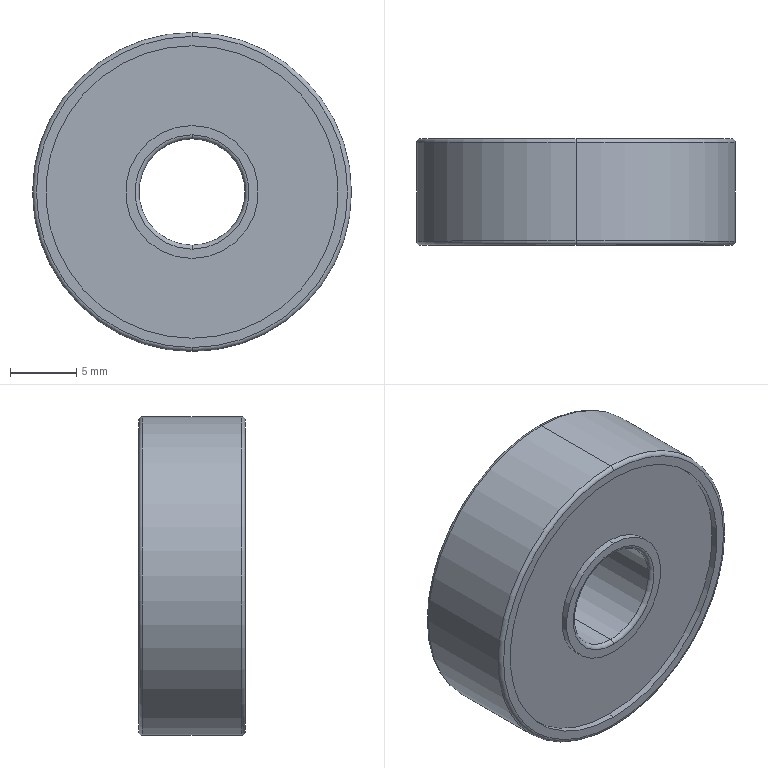Part | STEP file | Domestic miniature ball bearing NSK 628ZZ-1 | 1 solid | 26 faces | box 24 x 8 x 24 mm | volume 2912 mm3 | cylinder 12 | torus 8 | plane 6 | commonest cylinder face diameters 10 x4 22 x4 8 x2 24 x2
STEP:
#1=CARTESIAN_POINT('',(0.,24.998,-12.));
#2=VERTEX_POINT('',#1);
#3=CARTESIAN_POINT('',(0.,24.998,12.));
#4=VERTEX_POINT('',#3);
#5=CARTESIAN_POINT('',(0.,24.998,0.));
#6=DIRECTION('',(0.,-1.,0.));
#7=DIRECTION('',(0.,0.,1.));
#8=AXIS2_PLACEMENT_3D('',#5,#6,#7);
#9=CIRCLE('',#8,12.);
#10=EDGE_CURVE('',#2,#4,#9,.T.);
#11=ORIENTED_EDGE('',*,*,#10,.F.);
#12=CARTESIAN_POINT('',(0.,25.298,-11.7));
#13=VERTEX_POINT('',#12);
#14=CARTESIAN_POINT('',(0.,24.998,-11.7));
#15=DIRECTION('',(1.,0.,0.));
#16=DIRECTION('',(0.,0.,-1.));
#17=AXIS2_PLACEMENT_3D('',#14,#15,#16);
#18=CIRCLE('',#17,0.3);
#19=EDGE_CURVE('',#2,#13,#18,.T.);
#20=ORIENTED_EDGE('',*,*,#19,.T.);
#21=CARTESIAN_POINT('',(0.,25.298,11.7));
#22=VERTEX_POINT('',#21);
#23=CARTESIAN_POINT('',(0.,25.298,0.));
#24=DIRECTION('',(0.,1.,0.));
#25=DIRECTION('',(0.,0.,1.));
#26=AXIS2_PLACEMENT_3D('',#23,#24,#25);
#27=CIRCLE('',#26,11.7);
#28=EDGE_CURVE('',#22,#13,#27,.T.);
#29=ORIENTED_EDGE('',*,*,#28,.F.);
#30=CARTESIAN_POINT('',(0.,24.998,11.7));
#31=DIRECTION('',(-1.,0.,0.));
#32=DIRECTION('',(0.,0.,1.));
#33=AXIS2_PLACEMENT_3D('',#30,#31,#32);
#34=CIRCLE('',#33,0.3);
#35=EDGE_CURVE('',#4,#22,#34,.T.);
#36=ORIENTED_EDGE('',*,*,#35,.F.);
#37=EDGE_LOOP('',(#11,#20,#29,#36));
#38=FACE_OUTER_BOUND('',#37,.T.);
#39=CARTESIAN_POINT('',(0.,24.998,0.));
#40=DIRECTION('',(0.,1.,0.));
#41=DIRECTION('',(0.,0.,1.));
#42=AXIS2_PLACEMENT_3D('',#39,#40,#41);
#43=TOROIDAL_SURFACE('',#42,11.7,0.3);
#44=ADVANCED_FACE('',(#38),#43,.T.);
#45=CARTESIAN_POINT('',(0.,17.598,12.));
#46=VERTEX_POINT('',#45);
#47=CARTESIAN_POINT('',(0.,17.598,-12.));
#48=VERTEX_POINT('',#47);
#49=CARTESIAN_POINT('',(0.,17.598,0.));
#50=DIRECTION('',(0.,1.,0.));
#51=DIRECTION('',(0.,0.,-1.));
#52=AXIS2_PLACEMENT_3D('',#49,#50,#51);
#53=CIRCLE('',#52,12.);
#54=EDGE_CURVE('',#46,#48,#53,.T.);
#55=ORIENTED_EDGE('',*,*,#54,.F.);
#56=CARTESIAN_POINT('',(0.,17.298,11.7));
#57=VERTEX_POINT('',#56);
#58=CARTESIAN_POINT('',(0.,17.598,11.7));
#59=DIRECTION('',(1.,0.,0.));
#60=DIRECTION('',(0.,0.,-1.));
#61=AXIS2_PLACEMENT_3D('',#58,#59,#60);
#62=CIRCLE('',#61,0.3);
#63=EDGE_CURVE('',#46,#57,#62,.T.);
#64=ORIENTED_EDGE('',*,*,#63,.T.);
#65=CARTESIAN_POINT('',(0.,17.298,-11.7));
#66=VERTEX_POINT('',#65);
#67=CARTESIAN_POINT('',(0.,17.298,0.));
#68=DIRECTION('',(0.,-1.,0.));
#69=DIRECTION('',(0.,0.,-1.));
#70=AXIS2_PLACEMENT_3D('',#67,#68,#69);
#71=CIRCLE('',#70,11.7);
#72=EDGE_CURVE('',#66,#57,#71,.T.);
#73=ORIENTED_EDGE('',*,*,#72,.F.);
#74=CARTESIAN_POINT('',(0.,17.598,-11.7));
#75=DIRECTION('',(-1.,0.,0.));
#76=DIRECTION('',(0.,0.,1.));
#77=AXIS2_PLACEMENT_3D('',#74,#75,#76);
#78=CIRCLE('',#77,0.3);
#79=EDGE_CURVE('',#48,#66,#78,.T.);
#80=ORIENTED_EDGE('',*,*,#79,.F.);
#81=EDGE_LOOP('',(#55,#64,#73,#80));
#82=FACE_OUTER_BOUND('',#81,.T.);
#83=CARTESIAN_POINT('',(0.,17.598,0.));
#84=DIRECTION('',(0.,-1.,0.));
#85=DIRECTION('',(0.,0.,-1.));
#86=AXIS2_PLACEMENT_3D('',#83,#84,#85);
#87=TOROIDAL_SURFACE('',#86,11.7,0.3);
#88=ADVANCED_FACE('',(#82),#87,.T.);
#89=CARTESIAN_POINT('',(0.,25.298,-4.3));
#90=VERTEX_POINT('',#89);
#91=CARTESIAN_POINT('',(0.,25.298,4.3));
#92=VERTEX_POINT('',#91);
#93=CARTESIAN_POINT('',(0.,25.298,0.));
#94=DIRECTION('',(0.,-1.,0.));
#95=DIRECTION('',(0.,0.,1.));
#96=AXIS2_PLACEMENT_3D('',#93,#94,#95);
#97=CIRCLE('',#96,4.3);
#98=EDGE_CURVE('',#90,#92,#97,.T.);
#99=ORIENTED_EDGE('',*,*,#98,.F.);
#100=CARTESIAN_POINT('',(0.,24.998,-4.));
#101=VERTEX_POINT('',#100);
#102=CARTESIAN_POINT('',(0.,24.998,-4.3));
#103=DIRECTION('',(1.,0.,0.));
#104=DIRECTION('',(0.,0.,-1.));
#105=AXIS2_PLACEMENT_3D('',#102,#103,#104);
#106=CIRCLE('',#105,0.3);
#107=EDGE_CURVE('',#90,#101,#106,.T.);
#108=ORIENTED_EDGE('',*,*,#107,.T.);
#109=CARTESIAN_POINT('',(0.,24.998,4.));
#110=VERTEX_POINT('',#109);
#111=CARTESIAN_POINT('',(0.,24.998,0.));
#112=DIRECTION('',(0.,1.,0.));
#113=DIRECTION('',(0.,0.,1.));
#114=AXIS2_PLACEMENT_3D('',#111,#112,#113);
#115=CIRCLE('',#114,4.);
#116=EDGE_CURVE('',#110,#101,#115,.T.);
#117=ORIENTED_EDGE('',*,*,#116,.F.);
#118=CARTESIAN_POINT('',(0.,24.998,4.3));
#119=DIRECTION('',(-1.,0.,0.));
#120=DIRECTION('',(0.,0.,1.));
#121=AXIS2_PLACEMENT_3D('',#118,#119,#120);
#122=CIRCLE('',#121,0.3);
#123=EDGE_CURVE('',#92,#110,#122,.T.);
#124=ORIENTED_EDGE('',*,*,#123,.F.);
#125=EDGE_LOOP('',(#99,#108,#117,#124));
#126=FACE_OUTER_BOUND('',#125,.T.);
#127=CARTESIAN_POINT('',(0.,24.998,0.));
#128=DIRECTION('',(0.,1.,0.));
#129=DIRECTION('',(0.,0.,1.));
#130=AXIS2_PLACEMENT_3D('',#127,#128,#129);
#131=TOROIDAL_SURFACE('',#130,4.3,0.3);
#132=ADVANCED_FACE('',(#126),#131,.T.);
#133=CARTESIAN_POINT('',(0.,17.298,4.3));
#134=VERTEX_POINT('',#133);
#135=CARTESIAN_POINT('',(0.,17.298,-4.3));
#136=VERTEX_POINT('',#135);
#137=CARTESIAN_POINT('',(0.,17.298,0.));
#138=DIRECTION('',(0.,1.,0.));
#139=DIRECTION('',(0.,0.,-1.));
#140=AXIS2_PLACEMENT_3D('',#137,#138,#139);
#141=CIRCLE('',#140,4.3);
#142=EDGE_CURVE('',#134,#136,#141,.T.);
#143=ORIENTED_EDGE('',*,*,#142,.F.);
#144=CARTESIAN_POINT('',(0.,17.598,4.));
#145=VERTEX_POINT('',#144);
#146=CARTESIAN_POINT('',(0.,17.598,4.3));
#147=DIRECTION('',(1.,0.,0.));
#148=DIRECTION('',(0.,0.,-1.));
#149=AXIS2_PLACEMENT_3D('',#146,#147,#148);
#150=CIRCLE('',#149,0.3);
#151=EDGE_CURVE('',#134,#145,#150,.T.);
#152=ORIENTED_EDGE('',*,*,#151,.T.);
#153=CARTESIAN_POINT('',(0.,17.598,-4.));
#154=VERTEX_POINT('',#153);
#155=CARTESIAN_POINT('',(0.,17.598,0.));
#156=DIRECTION('',(0.,-1.,0.));
#157=DIRECTION('',(0.,0.,-1.));
#158=AXIS2_PLACEMENT_3D('',#155,#156,#157);
#159=CIRCLE('',#158,4.);
#160=EDGE_CURVE('',#154,#145,#159,.T.);
#161=ORIENTED_EDGE('',*,*,#160,.F.);
#162=CARTESIAN_POINT('',(0.,17.598,-4.3));
#163=DIRECTION('',(-1.,0.,0.));
#164=DIRECTION('',(0.,0.,1.));
#165=AXIS2_PLACEMENT_3D('',#162,#163,#164);
#166=CIRCLE('',#165,0.3);
#167=EDGE_CURVE('',#136,#154,#166,.T.);
#168=ORIENTED_EDGE('',*,*,#167,.F.);
#169=EDGE_LOOP('',(#143,#152,#161,#168));
#170=FACE_OUTER_BOUND('',#169,.T.);
#171=CARTESIAN_POINT('',(0.,17.598,0.));
#172=DIRECTION('',(0.,-1.,0.));
#173=DIRECTION('',(0.,0.,-1.));
#174=AXIS2_PLACEMENT_3D('',#171,#172,#173);
#175=TOROIDAL_SURFACE('',#174,4.3,0.3);
#176=ADVANCED_FACE('',(#170),#175,.T.);
#177=CARTESIAN_POINT('',(0.,25.298,-5.));
#178=VERTEX_POINT('',#177);
#179=CARTESIAN_POINT('',(0.,25.298,5.));
#180=VERTEX_POINT('',#179);
#181=CARTESIAN_POINT('',(0.,25.298,0.));
#182=DIRECTION('',(0.,-1.,0.));
#183=DIRECTION('',(0.,0.,-1.));
#184=AXIS2_PLACEMENT_3D('',#181,#182,#183);
#185=CIRCLE('',#184,5.);
#186=EDGE_CURVE('',#178,#180,#185,.T.);
#187=ORIENTED_EDGE('',*,*,#186,.T.);
#188=CARTESIAN_POINT('',(0.,24.798,5.));
#189=VERTEX_POINT('',#188);
#190=CARTESIAN_POINT('',(0.,0.,5.));
#191=DIRECTION('',(0.,-1.,0.));
#192=VECTOR('',#191,1000.);
#193=LINE('',#190,#192);
#194=EDGE_CURVE('',#180,#189,#193,.T.);
#195=ORIENTED_EDGE('',*,*,#194,.T.);
#196=CARTESIAN_POINT('',(0.,24.798,-5.));
#197=VERTEX_POINT('',#196);
#198=CARTESIAN_POINT('',(0.,24.798,0.));
#199=DIRECTION('',(0.,-1.,0.));
#200=DIRECTION('',(0.,0.,-1.));
#201=AXIS2_PLACEMENT_3D('',#198,#199,#200);
#202=CIRCLE('',#201,5.);
#203=EDGE_CURVE('',#197,#189,#202,.T.);
#204=ORIENTED_EDGE('',*,*,#203,.F.);
#205=CARTESIAN_POINT('',(0.,0.,-5.));
#206=DIRECTION('',(0.,-1.,0.));
#207=VECTOR('',#206,1000.);
#208=LINE('',#205,#207);
#209=EDGE_CURVE('',#178,#197,#208,.T.);
#210=ORIENTED_EDGE('',*,*,#209,.F.);
#211=EDGE_LOOP('',(#187,#195,#204,#210));
#212=FACE_OUTER_BOUND('',#211,.T.);
#213=CARTESIAN_POINT('',(0.,0.,0.));
#214=DIRECTION('',(0.,-1.,0.));
#215=DIRECTION('',(0.,0.,-1.));
#216=AXIS2_PLACEMENT_3D('',#213,#214,#215);
#217=CYLINDRICAL_SURFACE('',#216,5.);
#218=ADVANCED_FACE('',(#212),#217,.T.);
#219=CARTESIAN_POINT('',(0.,25.298,11.));
#220=VERTEX_POINT('',#219);
#221=CARTESIAN_POINT('',(0.,25.298,-11.));
#222=VERTEX_POINT('',#221);
#223=CARTESIAN_POINT('',(0.,25.298,0.));
#224=DIRECTION('',(0.,-1.,0.));
#225=DIRECTION('',(0.,0.,-1.));
#226=AXIS2_PLACEMENT_3D('',#223,#224,#225);
#227=CIRCLE('',#226,11.);
#228=EDGE_CURVE('',#220,#222,#227,.T.);
#229=ORIENTED_EDGE('',*,*,#228,.F.);
#230=CARTESIAN_POINT('',(0.,24.798,11.));
#231=VERTEX_POINT('',#230);
#232=CARTESIAN_POINT('',(0.,0.,11.));
#233=DIRECTION('',(0.,-1.,0.));
#234=VECTOR('',#233,1000.);
#235=LINE('',#232,#234);
#236=EDGE_CURVE('',#220,#231,#235,.T.);
#237=ORIENTED_EDGE('',*,*,#236,.T.);
#238=CARTESIAN_POINT('',(0.,24.798,-11.));
#239=VERTEX_POINT('',#238);
#240=CARTESIAN_POINT('',(0.,24.798,0.));
#241=DIRECTION('',(0.,-1.,0.));
#242=DIRECTION('',(0.,0.,-1.));
#243=AXIS2_PLACEMENT_3D('',#240,#241,#242);
#244=CIRCLE('',#243,11.);
#245=EDGE_CURVE('',#231,#239,#244,.T.);
#246=ORIENTED_EDGE('',*,*,#245,.T.);
#247=CARTESIAN_POINT('',(0.,0.,-11.));
#248=DIRECTION('',(0.,-1.,0.));
#249=VECTOR('',#248,1000.);
#250=LINE('',#247,#249);
#251=EDGE_CURVE('',#222,#239,#250,.T.);
#252=ORIENTED_EDGE('',*,*,#251,.F.);
#253=EDGE_LOOP('',(#229,#237,#246,#252));
#254=FACE_OUTER_BOUND('',#253,.T.);
#255=CARTESIAN_POINT('',(0.,0.,0.));
#256=DIRECTION('',(0.,-1.,0.));
#257=DIRECTION('',(0.,0.,-1.));
#258=AXIS2_PLACEMENT_3D('',#255,#256,#257);
#259=CYLINDRICAL_SURFACE('',#258,11.);
#260=ADVANCED_FACE('',(#254),#259,.F.);
#261=ORIENTED_EDGE('',*,*,#10,.T.);
#262=CARTESIAN_POINT('',(0.,0.,12.));
#263=DIRECTION('',(0.,-1.,0.));
#264=VECTOR('',#263,1000.);
#265=LINE('',#262,#264);
#266=EDGE_CURVE('',#4,#46,#265,.T.);
#267=ORIENTED_EDGE('',*,*,#266,.T.);
#268=ORIENTED_EDGE('',*,*,#54,.T.);
#269=CARTESIAN_POINT('',(0.,0.,-12.));
#270=DIRECTION('',(0.,-1.,0.));
#271=VECTOR('',#270,1000.);
#272=LINE('',#269,#271);
#273=EDGE_CURVE('',#2,#48,#272,.T.);
#274=ORIENTED_EDGE('',*,*,#273,.F.);
#275=EDGE_LOOP('',(#261,#267,#268,#274));
#276=FACE_OUTER_BOUND('',#275,.T.);
#277=CARTESIAN_POINT('',(0.,0.,0.));
#278=DIRECTION('',(0.,-1.,0.));
#279=DIRECTION('',(0.,0.,-1.));
#280=AXIS2_PLACEMENT_3D('',#277,#278,#279);
#281=CYLINDRICAL_SURFACE('',#280,12.);
#282=ADVANCED_FACE('',(#276),#281,.T.);
#283=CARTESIAN_POINT('',(0.,17.798,11.));
#284=VERTEX_POINT('',#283);
#285=CARTESIAN_POINT('',(0.,17.798,-11.));
#286=VERTEX_POINT('',#285);
#287=CARTESIAN_POINT('',(0.,17.798,0.));
#288=DIRECTION('',(0.,-1.,0.));
#289=DIRECTION('',(0.,0.,-1.));
#290=AXIS2_PLACEMENT_3D('',#287,#288,#289);
#291=CIRCLE('',#290,11.);
#292=EDGE_CURVE('',#284,#286,#291,.T.);
#293=ORIENTED_EDGE('',*,*,#292,.F.);
#294=CARTESIAN_POINT('',(0.,17.298,11.));
#295=VERTEX_POINT('',#294);
#296=CARTESIAN_POINT('',(0.,0.,11.));
#297=DIRECTION('',(0.,-1.,0.));
#298=VECTOR('',#297,1000.);
#299=LINE('',#296,#298);
#300=EDGE_CURVE('',#284,#295,#299,.T.);
#301=ORIENTED_EDGE('',*,*,#300,.T.);
#302=CARTESIAN_POINT('',(0.,17.298,-11.));
#303=VERTEX_POINT('',#302);
#304=CARTESIAN_POINT('',(0.,17.298,0.));
#305=DIRECTION('',(0.,-1.,0.));
#306=DIRECTION('',(0.,0.,-1.));
#307=AXIS2_PLACEMENT_3D('',#304,#305,#306);
#308=CIRCLE('',#307,11.);
#309=EDGE_CURVE('',#295,#303,#308,.T.);
#310=ORIENTED_EDGE('',*,*,#309,.T.);
#311=CARTESIAN_POINT('',(0.,0.,-11.));
#312=DIRECTION('',(0.,-1.,0.));
#313=VECTOR('',#312,1000.);
#314=LINE('',#311,#313);
#315=EDGE_CURVE('',#286,#303,#314,.T.);
#316=ORIENTED_EDGE('',*,*,#315,.F.);
#317=EDGE_LOOP('',(#293,#301,#310,#316));
#318=FACE_OUTER_BOUND('',#317,.T.);
#319=CARTESIAN_POINT('',(0.,0.,0.));
#320=DIRECTION('',(0.,-1.,0.));
#321=DIRECTION('',(0.,0.,-1.));
#322=AXIS2_PLACEMENT_3D('',#319,#320,#321);
#323=CYLINDRICAL_SURFACE('',#322,11.);
#324=ADVANCED_FACE('',(#318),#323,.F.);
#325=CARTESIAN_POINT('',(0.,17.798,-5.));
#326=VERTEX_POINT('',#325);
#327=CARTESIAN_POINT('',(0.,17.798,5.));
#328=VERTEX_POINT('',#327);
#329=CARTESIAN_POINT('',(0.,17.798,0.));
#330=DIRECTION('',(0.,-1.,0.));
#331=DIRECTION('',(0.,0.,-1.));
#332=AXIS2_PLACEMENT_3D('',#329,#330,#331);
#333=CIRCLE('',#332,5.);
#334=EDGE_CURVE('',#326,#328,#333,.T.);
#335=ORIENTED_EDGE('',*,*,#334,.T.);
#336=CARTESIAN_POINT('',(0.,17.298,5.));
#337=VERTEX_POINT('',#336);
#338=CARTESIAN_POINT('',(0.,0.,5.));
#339=DIRECTION('',(0.,-1.,0.));
#340=VECTOR('',#339,1000.);
#341=LINE('',#338,#340);
#342=EDGE_CURVE('',#328,#337,#341,.T.);
#343=ORIENTED_EDGE('',*,*,#342,.T.);
#344=CARTESIAN_POINT('',(0.,17.298,-5.));
#345=VERTEX_POINT('',#344);
#346=CARTESIAN_POINT('',(0.,17.298,0.));
#347=DIRECTION('',(0.,-1.,0.));
#348=DIRECTION('',(0.,0.,-1.));
#349=AXIS2_PLACEMENT_3D('',#346,#347,#348);
#350=CIRCLE('',#349,5.);
#351=EDGE_CURVE('',#345,#337,#350,.T.);
#352=ORIENTED_EDGE('',*,*,#351,.F.);
#353=CARTESIAN_POINT('',(0.,0.,-5.));
#354=DIRECTION('',(0.,-1.,0.));
#355=VECTOR('',#354,1000.);
#356=LINE('',#353,#355);
#357=EDGE_CURVE('',#326,#345,#356,.T.);
#358=ORIENTED_EDGE('',*,*,#357,.F.);
#359=EDGE_LOOP('',(#335,#343,#352,#358));
#360=FACE_OUTER_BOUND('',#359,.T.);
#361=CARTESIAN_POINT('',(0.,0.,0.));
#362=DIRECTION('',(0.,-1.,0.));
#363=DIRECTION('',(0.,0.,-1.));
#364=AXIS2_PLACEMENT_3D('',#361,#362,#363);
#365=CYLINDRICAL_SURFACE('',#364,5.);
#366=ADVANCED_FACE('',(#360),#365,.T.);
#367=CARTESIAN_POINT('',(0.,24.998,0.));
#368=DIRECTION('',(0.,1.,0.));
#369=DIRECTION('',(0.,0.,1.));
#370=AXIS2_PLACEMENT_3D('',#367,#368,#369);
#371=CIRCLE('',#370,4.);
#372=EDGE_CURVE('',#101,#110,#371,.T.);
#373=ORIENTED_EDGE('',*,*,#372,.T.);
#374=CARTESIAN_POINT('',(0.,0.,4.));
#375=DIRECTION('',(0.,-1.,0.));
#376=VECTOR('',#375,1000.);
#377=LINE('',#374,#376);
#378=EDGE_CURVE('',#110,#145,#377,.T.);
#379=ORIENTED_EDGE('',*,*,#378,.T.);
#380=CARTESIAN_POINT('',(0.,17.598,0.));
#381=DIRECTION('',(0.,-1.,0.));
#382=DIRECTION('',(0.,0.,-1.));
#383=AXIS2_PLACEMENT_3D('',#380,#381,#382);
#384=CIRCLE('',#383,4.);
#385=EDGE_CURVE('',#145,#154,#384,.T.);
#386=ORIENTED_EDGE('',*,*,#385,.T.);
#387=CARTESIAN_POINT('',(0.,0.,-4.));
#388=DIRECTION('',(0.,-1.,0.));
#389=VECTOR('',#388,1000.);
#390=LINE('',#387,#389);
#391=EDGE_CURVE('',#101,#154,#390,.T.);
#392=ORIENTED_EDGE('',*,*,#391,.F.);
#393=EDGE_LOOP('',(#373,#379,#386,#392));
#394=FACE_OUTER_BOUND('',#393,.T.);
#395=CARTESIAN_POINT('',(0.,0.,0.));
#396=DIRECTION('',(0.,-1.,0.));
#397=DIRECTION('',(0.,0.,-1.));
#398=AXIS2_PLACEMENT_3D('',#395,#396,#397);
#399=CYLINDRICAL_SURFACE('',#398,4.);
#400=ADVANCED_FACE('',(#394),#399,.F.);
#401=CARTESIAN_POINT('',(0.,25.298,0.));
#402=DIRECTION('',(0.,-1.,0.));
#403=DIRECTION('',(0.,0.,1.));
#404=AXIS2_PLACEMENT_3D('',#401,#402,#403);
#405=CIRCLE('',#404,4.3);
#406=EDGE_CURVE('',#92,#90,#405,.T.);
#407=ORIENTED_EDGE('',*,*,#406,.T.);
#408=ORIENTED_EDGE('',*,*,#98,.T.);
#409=EDGE_LOOP('',(#407,#408));
#410=FACE_BOUND('',#409,.T.);
#411=ORIENTED_EDGE('',*,*,#186,.F.);
#412=CARTESIAN_POINT('',(0.,25.298,0.));
#413=DIRECTION('',(0.,-1.,0.));
#414=DIRECTION('',(0.,0.,-1.));
#415=AXIS2_PLACEMENT_3D('',#412,#413,#414);
#416=CIRCLE('',#415,5.);
#417=EDGE_CURVE('',#180,#178,#416,.T.);
#418=ORIENTED_EDGE('',*,*,#417,.F.);
#419=EDGE_LOOP('',(#411,#418));
#420=FACE_OUTER_BOUND('',#419,.T.);
#421=CARTESIAN_POINT('',(5.,25.298,0.));
#422=DIRECTION('',(0.,1.,0.));
#423=DIRECTION('',(0.,0.,1.));
#424=AXIS2_PLACEMENT_3D('',#421,#422,#423);
#425=PLANE('',#424);
#426=ADVANCED_FACE('',(#410,#420),#425,.T.);
#427=ORIENTED_EDGE('',*,*,#378,.F.);
#428=ORIENTED_EDGE('',*,*,#116,.T.);
#429=ORIENTED_EDGE('',*,*,#391,.T.);
#430=ORIENTED_EDGE('',*,*,#160,.T.);
#431=EDGE_LOOP('',(#427,#428,#429,#430));
#432=FACE_OUTER_BOUND('',#431,.T.);
#433=CARTESIAN_POINT('',(0.,0.,0.));
#434=DIRECTION('',(0.,-1.,0.));
#435=DIRECTION('',(0.,0.,-1.));
#436=AXIS2_PLACEMENT_3D('',#433,#434,#435);
#437=CYLINDRICAL_SURFACE('',#436,4.);
#438=ADVANCED_FACE('',(#432),#437,.F.);
#439=CARTESIAN_POINT('',(0.,17.298,0.));
#440=DIRECTION('',(0.,1.,0.));
#441=DIRECTION('',(0.,0.,-1.));
#442=AXIS2_PLACEMENT_3D('',#439,#440,#441);
#443=CIRCLE('',#442,4.3);
#444=EDGE_CURVE('',#136,#134,#443,.T.);
#445=ORIENTED_EDGE('',*,*,#444,.T.);
#446=ORIENTED_EDGE('',*,*,#142,.T.);
#447=EDGE_LOOP('',(#445,#446));
#448=FACE_BOUND('',#447,.T.);
#449=ORIENTED_EDGE('',*,*,#351,.T.);
#450=CARTESIAN_POINT('',(0.,17.298,0.));
#451=DIRECTION('',(0.,-1.,0.));
#452=DIRECTION('',(0.,0.,-1.));
#453=AXIS2_PLACEMENT_3D('',#450,#451,#452);
#454=CIRCLE('',#453,5.);
#455=EDGE_CURVE('',#337,#345,#454,.T.);
#456=ORIENTED_EDGE('',*,*,#455,.T.);
#457=EDGE_LOOP('',(#449,#456));
#458=FACE_OUTER_BOUND('',#457,.T.);
#459=CARTESIAN_POINT('',(4.,17.298,0.));
#460=DIRECTION('',(0.,-1.,0.));
#461=DIRECTION('',(0.,0.,-1.));
#462=AXIS2_PLACEMENT_3D('',#459,#460,#461);
#463=PLANE('',#462);
#464=ADVANCED_FACE('',(#448,#458),#463,.T.);
#465=ORIENTED_EDGE('',*,*,#342,.F.);
#466=CARTESIAN_POINT('',(0.,17.798,0.));
#467=DIRECTION('',(0.,-1.,0.));
#468=DIRECTION('',(0.,0.,-1.));
#469=AXIS2_PLACEMENT_3D('',#466,#467,#468);
#470=CIRCLE('',#469,5.);
#471=EDGE_CURVE('',#328,#326,#470,.T.);
#472=ORIENTED_EDGE('',*,*,#471,.T.);
#473=ORIENTED_EDGE('',*,*,#357,.T.);
#474=ORIENTED_EDGE('',*,*,#455,.F.);
#475=EDGE_LOOP('',(#465,#472,#473,#474));
#476=FACE_OUTER_BOUND('',#475,.T.);
#477=CARTESIAN_POINT('',(0.,0.,0.));
#478=DIRECTION('',(0.,-1.,0.));
#479=DIRECTION('',(0.,0.,-1.));
#480=AXIS2_PLACEMENT_3D('',#477,#478,#479);
#481=CYLINDRICAL_SURFACE('',#480,5.);
#482=ADVANCED_FACE('',(#476),#481,.T.);
#483=CARTESIAN_POINT('',(0.,17.798,0.));
#484=DIRECTION('',(0.,-1.,0.));
#485=DIRECTION('',(0.,0.,-1.));
#486=AXIS2_PLACEMENT_3D('',#483,#484,#485);
#487=CIRCLE('',#486,11.);
#488=EDGE_CURVE('',#286,#284,#487,.T.);
#489=ORIENTED_EDGE('',*,*,#488,.T.);
#490=ORIENTED_EDGE('',*,*,#292,.T.);
#491=EDGE_LOOP('',(#489,#490));
#492=FACE_OUTER_BOUND('',#491,.T.);
#493=ORIENTED_EDGE('',*,*,#334,.F.);
#494=ORIENTED_EDGE('',*,*,#471,.F.);
#495=EDGE_LOOP('',(#493,#494));
#496=FACE_BOUND('',#495,.T.);
#497=CARTESIAN_POINT('',(5.,17.798,0.));
#498=DIRECTION('',(0.,-1.,0.));
#499=DIRECTION('',(0.,0.,-1.));
#500=AXIS2_PLACEMENT_3D('',#497,#498,#499);
#501=PLANE('',#500);
#502=ADVANCED_FACE('',(#492,#496),#501,.T.);
#503=ORIENTED_EDGE('',*,*,#300,.F.);
#504=ORIENTED_EDGE('',*,*,#488,.F.);
#505=ORIENTED_EDGE('',*,*,#315,.T.);
#506=CARTESIAN_POINT('',(0.,17.298,0.));
#507=DIRECTION('',(0.,-1.,0.));
#508=DIRECTION('',(0.,0.,-1.));
#509=AXIS2_PLACEMENT_3D('',#506,#507,#508);
#510=CIRCLE('',#509,11.);
#511=EDGE_CURVE('',#303,#295,#510,.T.);
#512=ORIENTED_EDGE('',*,*,#511,.T.);
#513=EDGE_LOOP('',(#503,#504,#505,#512));
#514=FACE_OUTER_BOUND('',#513,.T.);
#515=CARTESIAN_POINT('',(0.,0.,0.));
#516=DIRECTION('',(0.,-1.,0.));
#517=DIRECTION('',(0.,0.,-1.));
#518=AXIS2_PLACEMENT_3D('',#515,#516,#517);
#519=CYLINDRICAL_SURFACE('',#518,11.);
#520=ADVANCED_FACE('',(#514),#519,.F.);
#521=ORIENTED_EDGE('',*,*,#72,.T.);
#522=CARTESIAN_POINT('',(0.,17.298,0.));
#523=DIRECTION('',(0.,-1.,0.));
#524=DIRECTION('',(0.,0.,-1.));
#525=AXIS2_PLACEMENT_3D('',#522,#523,#524);
#526=CIRCLE('',#525,11.7);
#527=EDGE_CURVE('',#57,#66,#526,.T.);
#528=ORIENTED_EDGE('',*,*,#527,.T.);
#529=EDGE_LOOP('',(#521,#528));
#530=FACE_OUTER_BOUND('',#529,.T.);
#531=ORIENTED_EDGE('',*,*,#511,.F.);
#532=ORIENTED_EDGE('',*,*,#309,.F.);
#533=EDGE_LOOP('',(#531,#532));
#534=FACE_BOUND('',#533,.T.);
#535=CARTESIAN_POINT('',(11.,17.298,0.));
#536=DIRECTION('',(0.,-1.,0.));
#537=DIRECTION('',(0.,0.,-1.));
#538=AXIS2_PLACEMENT_3D('',#535,#536,#537);
#539=PLANE('',#538);
#540=ADVANCED_FACE('',(#530,#534),#539,.T.);
#541=ORIENTED_EDGE('',*,*,#266,.F.);
#542=CARTESIAN_POINT('',(0.,24.998,0.));
#543=DIRECTION('',(0.,-1.,0.));
#544=DIRECTION('',(0.,0.,1.));
#545=AXIS2_PLACEMENT_3D('',#542,#543,#544);
#546=CIRCLE('',#545,12.);
#547=EDGE_CURVE('',#4,#2,#546,.T.);
#548=ORIENTED_EDGE('',*,*,#547,.T.);
#549=ORIENTED_EDGE('',*,*,#273,.T.);
#550=CARTESIAN_POINT('',(0.,17.598,0.));
#551=DIRECTION('',(0.,1.,0.));
#552=DIRECTION('',(0.,0.,-1.));
#553=AXIS2_PLACEMENT_3D('',#550,#551,#552);
#554=CIRCLE('',#553,12.);
#555=EDGE_CURVE('',#48,#46,#554,.T.);
#556=ORIENTED_EDGE('',*,*,#555,.T.);
#557=EDGE_LOOP('',(#541,#548,#549,#556));
#558=FACE_OUTER_BOUND('',#557,.T.);
#559=CARTESIAN_POINT('',(0.,0.,0.));
#560=DIRECTION('',(0.,-1.,0.));
#561=DIRECTION('',(0.,0.,-1.));
#562=AXIS2_PLACEMENT_3D('',#559,#560,#561);
#563=CYLINDRICAL_SURFACE('',#562,12.);
#564=ADVANCED_FACE('',(#558),#563,.T.);
#565=ORIENTED_EDGE('',*,*,#28,.T.);
#566=CARTESIAN_POINT('',(0.,25.298,0.));
#567=DIRECTION('',(0.,1.,0.));
#568=DIRECTION('',(0.,0.,1.));
#569=AXIS2_PLACEMENT_3D('',#566,#567,#568);
#570=CIRCLE('',#569,11.7);
#571=EDGE_CURVE('',#13,#22,#570,.T.);
#572=ORIENTED_EDGE('',*,*,#571,.T.);
#573=EDGE_LOOP('',(#565,#572));
#574=FACE_OUTER_BOUND('',#573,.T.);
#575=CARTESIAN_POINT('',(0.,25.298,0.));
#576=DIRECTION('',(0.,-1.,0.));
#577=DIRECTION('',(0.,0.,-1.));
#578=AXIS2_PLACEMENT_3D('',#575,#576,#577);
#579=CIRCLE('',#578,11.);
#580=EDGE_CURVE('',#222,#220,#579,.T.);
#581=ORIENTED_EDGE('',*,*,#580,.T.);
#582=ORIENTED_EDGE('',*,*,#228,.T.);
#583=EDGE_LOOP('',(#581,#582));
#584=FACE_BOUND('',#583,.T.);
#585=CARTESIAN_POINT('',(12.,25.298,0.));
#586=DIRECTION('',(0.,1.,0.));
#587=DIRECTION('',(0.,0.,1.));
#588=AXIS2_PLACEMENT_3D('',#585,#586,#587);
#589=PLANE('',#588);
#590=ADVANCED_FACE('',(#574,#584),#589,.T.);
#591=ORIENTED_EDGE('',*,*,#236,.F.);
#592=ORIENTED_EDGE('',*,*,#580,.F.);
#593=ORIENTED_EDGE('',*,*,#251,.T.);
#594=CARTESIAN_POINT('',(0.,24.798,0.));
#595=DIRECTION('',(0.,-1.,0.));
#596=DIRECTION('',(0.,0.,-1.));
#597=AXIS2_PLACEMENT_3D('',#594,#595,#596);
#598=CIRCLE('',#597,11.);
#599=EDGE_CURVE('',#239,#231,#598,.T.);
#600=ORIENTED_EDGE('',*,*,#599,.T.);
#601=EDGE_LOOP('',(#591,#592,#593,#600));
#602=FACE_OUTER_BOUND('',#601,.T.);
#603=CARTESIAN_POINT('',(0.,0.,0.));
#604=DIRECTION('',(0.,-1.,0.));
#605=DIRECTION('',(0.,0.,-1.));
#606=AXIS2_PLACEMENT_3D('',#603,#604,#605);
#607=CYLINDRICAL_SURFACE('',#606,11.);
#608=ADVANCED_FACE('',(#602),#607,.F.);
#609=ORIENTED_EDGE('',*,*,#203,.T.);
#610=CARTESIAN_POINT('',(0.,24.798,0.));
#611=DIRECTION('',(0.,-1.,0.));
#612=DIRECTION('',(0.,0.,-1.));
#613=AXIS2_PLACEMENT_3D('',#610,#611,#612);
#614=CIRCLE('',#613,5.);
#615=EDGE_CURVE('',#189,#197,#614,.T.);
#616=ORIENTED_EDGE('',*,*,#615,.T.);
#617=EDGE_LOOP('',(#609,#616));
#618=FACE_BOUND('',#617,.T.);
#619=ORIENTED_EDGE('',*,*,#599,.F.);
#620=ORIENTED_EDGE('',*,*,#245,.F.);
#621=EDGE_LOOP('',(#619,#620));
#622=FACE_OUTER_BOUND('',#621,.T.);
#623=CARTESIAN_POINT('',(11.,24.798,0.));
#624=DIRECTION('',(0.,1.,0.));
#625=DIRECTION('',(0.,0.,1.));
#626=AXIS2_PLACEMENT_3D('',#623,#624,#625);
#627=PLANE('',#626);
#628=ADVANCED_FACE('',(#618,#622),#627,.T.);
#629=ORIENTED_EDGE('',*,*,#194,.F.);
#630=ORIENTED_EDGE('',*,*,#417,.T.);
#631=ORIENTED_EDGE('',*,*,#209,.T.);
#632=ORIENTED_EDGE('',*,*,#615,.F.);
#633=EDGE_LOOP('',(#629,#630,#631,#632));
#634=FACE_OUTER_BOUND('',#633,.T.);
#635=CARTESIAN_POINT('',(0.,0.,0.));
#636=DIRECTION('',(0.,-1.,0.));
#637=DIRECTION('',(0.,0.,-1.));
#638=AXIS2_PLACEMENT_3D('',#635,#636,#637);
#639=CYLINDRICAL_SURFACE('',#638,5.);
#640=ADVANCED_FACE('',(#634),#639,.T.);
#641=ORIENTED_EDGE('',*,*,#151,.F.);
#642=ORIENTED_EDGE('',*,*,#444,.F.);
#643=ORIENTED_EDGE('',*,*,#167,.T.);
#644=ORIENTED_EDGE('',*,*,#385,.F.);
#645=EDGE_LOOP('',(#641,#642,#643,#644));
#646=FACE_OUTER_BOUND('',#645,.T.);
#647=CARTESIAN_POINT('',(0.,17.598,0.));
#648=DIRECTION('',(0.,-1.,0.));
#649=DIRECTION('',(0.,0.,-1.));
#650=AXIS2_PLACEMENT_3D('',#647,#648,#649);
#651=TOROIDAL_SURFACE('',#650,4.3,0.3);
#652=ADVANCED_FACE('',(#646),#651,.T.);
#653=ORIENTED_EDGE('',*,*,#107,.F.);
#654=ORIENTED_EDGE('',*,*,#406,.F.);
#655=ORIENTED_EDGE('',*,*,#123,.T.);
#656=ORIENTED_EDGE('',*,*,#372,.F.);
#657=EDGE_LOOP('',(#653,#654,#655,#656));
#658=FACE_OUTER_BOUND('',#657,.T.);
#659=CARTESIAN_POINT('',(0.,24.998,0.));
#660=DIRECTION('',(0.,1.,0.));
#661=DIRECTION('',(0.,0.,1.));
#662=AXIS2_PLACEMENT_3D('',#659,#660,#661);
#663=TOROIDAL_SURFACE('',#662,4.3,0.3);
#664=ADVANCED_FACE('',(#658),#663,.T.);
#665=ORIENTED_EDGE('',*,*,#63,.F.);
#666=ORIENTED_EDGE('',*,*,#555,.F.);
#667=ORIENTED_EDGE('',*,*,#79,.T.);
#668=ORIENTED_EDGE('',*,*,#527,.F.);
#669=EDGE_LOOP('',(#665,#666,#667,#668));
#670=FACE_OUTER_BOUND('',#669,.T.);
#671=CARTESIAN_POINT('',(0.,17.598,0.));
#672=DIRECTION('',(0.,-1.,0.));
#673=DIRECTION('',(0.,0.,-1.));
#674=AXIS2_PLACEMENT_3D('',#671,#672,#673);
#675=TOROIDAL_SURFACE('',#674,11.7,0.3);
#676=ADVANCED_FACE('',(#670),#675,.T.);
#677=ORIENTED_EDGE('',*,*,#19,.F.);
#678=ORIENTED_EDGE('',*,*,#547,.F.);
#679=ORIENTED_EDGE('',*,*,#35,.T.);
#680=ORIENTED_EDGE('',*,*,#571,.F.);
#681=EDGE_LOOP('',(#677,#678,#679,#680));
#682=FACE_OUTER_BOUND('',#681,.T.);
#683=CARTESIAN_POINT('',(0.,24.998,0.));
#684=DIRECTION('',(0.,1.,0.));
#685=DIRECTION('',(0.,0.,1.));
#686=AXIS2_PLACEMENT_3D('',#683,#684,#685);
#687=TOROIDAL_SURFACE('',#686,11.7,0.3);
#688=ADVANCED_FACE('',(#682),#687,.T.);
#689=CLOSED_SHELL('',(#44,#88,#132,#176,#218,#260,#282,#324,#366,#400,#426,#438,#464,#482,#502,#520,#540,#564,#590,#608,#628,#640,#652,#664,#676,#688));
#690=MANIFOLD_SOLID_BREP('',#689);
#691=CARTESIAN_POINT('',(0.,0.,0.));
#692=DIRECTION('',(0.,0.,1.));
#693=DIRECTION('',(1.,0.,0.));
#694=AXIS2_PLACEMENT_3D('',#691,#692,#693);
#695=(LENGTH_UNIT()NAMED_UNIT(*)SI_UNIT(.MILLI.,.METRE.));
#696=UNCERTAINTY_MEASURE_WITH_UNIT(LENGTH_MEASURE(0.00001),#695,'','');
#697=(NAMED_UNIT(*)PLANE_ANGLE_UNIT()SI_UNIT($,.RADIAN.));
#698=(NAMED_UNIT(*)SI_UNIT($,.STERADIAN.)SOLID_ANGLE_UNIT());
#699=(GEOMETRIC_REPRESENTATION_CONTEXT(3)GLOBAL_UNCERTAINTY_ASSIGNED_CONTEXT((#696))GLOBAL_UNIT_ASSIGNED_CONTEXT((#695,#697,#698))REPRESENTATION_CONTEXT('',''));
#700=ADVANCED_BREP_SHAPE_REPRESENTATION('',(#690,#694),#699);